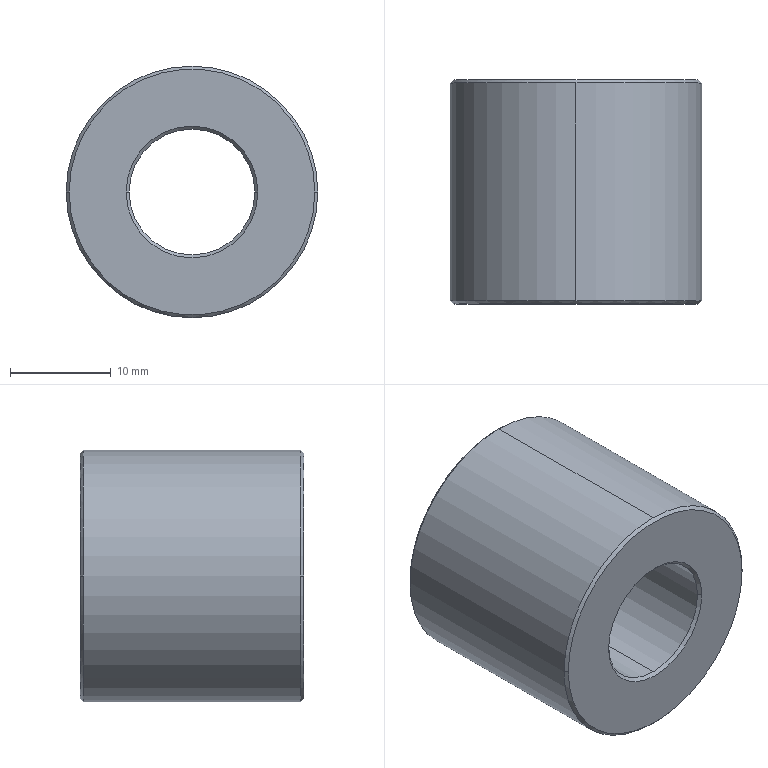Part | NX | 1 solid | 14 faces | box 25 x 22.25 x 25 mm | volume 8181 mm3 | cone 8 | cylinder 4 | plane 2 | commonest cylinder face diameters 12.5 x2 25 x2
STEP:
#1=CARTESIAN_POINT('',(12.5,-29.95,-71.));
#2=VERTEX_POINT('',#1);
#3=CARTESIAN_POINT('',(0.,-29.95,-83.5));
#4=VERTEX_POINT('',#3);
#5=CARTESIAN_POINT('',(0.,-29.95,-71.));
#6=DIRECTION('',(0.,1.,0.));
#7=DIRECTION('',(0.,0.,-1.));
#8=AXIS2_PLACEMENT_3D('',#5,#6,#7);
#9=CIRCLE('',#8,12.5);
#10=EDGE_CURVE('',#2,#4,#9,.T.);
#11=ORIENTED_EDGE('',*,*,#10,.T.);
#12=CARTESIAN_POINT('',(0.,-8.3,-83.5));
#13=VERTEX_POINT('',#12);
#14=CARTESIAN_POINT('',(0.,-30.25,-83.5));
#15=DIRECTION('',(0.,1.,0.));
#16=VECTOR('',#15,1000.);
#17=LINE('',#14,#16);
#18=EDGE_CURVE('',#13,#4,#17,.F.);
#19=ORIENTED_EDGE('',*,*,#18,.F.);
#20=CARTESIAN_POINT('',(12.5,-8.3,-71.));
#21=VERTEX_POINT('',#20);
#22=CARTESIAN_POINT('',(0.,-8.3,-71.));
#23=DIRECTION('',(0.,1.,0.));
#24=DIRECTION('',(0.,0.,-1.));
#25=AXIS2_PLACEMENT_3D('',#22,#23,#24);
#26=CIRCLE('',#25,12.5);
#27=EDGE_CURVE('',#21,#13,#26,.T.);
#28=ORIENTED_EDGE('',*,*,#27,.F.);
#29=CARTESIAN_POINT('',(0.,-8.3,-58.5));
#30=VERTEX_POINT('',#29);
#31=CARTESIAN_POINT('',(0.,-8.3,-71.));
#32=DIRECTION('',(0.,1.,0.));
#33=DIRECTION('',(0.,0.,-1.));
#34=AXIS2_PLACEMENT_3D('',#31,#32,#33);
#35=CIRCLE('',#34,12.5);
#36=EDGE_CURVE('',#30,#21,#35,.T.);
#37=ORIENTED_EDGE('',*,*,#36,.F.);
#38=CARTESIAN_POINT('',(0.,-29.95,-58.5));
#39=VERTEX_POINT('',#38);
#40=CARTESIAN_POINT('',(0.,-30.25,-58.5));
#41=DIRECTION('',(0.,1.,0.));
#42=VECTOR('',#41,1000.);
#43=LINE('',#40,#42);
#44=EDGE_CURVE('',#30,#39,#43,.F.);
#45=ORIENTED_EDGE('',*,*,#44,.T.);
#46=CARTESIAN_POINT('',(0.,-29.95,-71.));
#47=DIRECTION('',(0.,1.,0.));
#48=DIRECTION('',(0.,0.,-1.));
#49=AXIS2_PLACEMENT_3D('',#46,#47,#48);
#50=CIRCLE('',#49,12.5);
#51=EDGE_CURVE('',#39,#2,#50,.T.);
#52=ORIENTED_EDGE('',*,*,#51,.T.);
#53=EDGE_LOOP('',(#11,#19,#28,#37,#45,#52));
#54=FACE_BOUND('',#53,.T.);
#55=CARTESIAN_POINT('',(0.,-30.25,-71.));
#56=DIRECTION('',(0.,1.,0.));
#57=DIRECTION('',(0.,0.,-1.));
#58=AXIS2_PLACEMENT_3D('',#55,#56,#57);
#59=CYLINDRICAL_SURFACE('',#58,12.5);
#60=ADVANCED_FACE('',(#54),#59,.T.);
#61=ORIENTED_EDGE('',*,*,#10,.F.);
#62=CARTESIAN_POINT('',(12.2,-30.25,-71.));
#63=VERTEX_POINT('',#62);
#64=CARTESIAN_POINT('',(12.2,-30.25,-71.));
#65=DIRECTION('',(0.7071,0.7071,0.));
#66=VECTOR('',#65,1000.);
#67=LINE('',#64,#66);
#68=EDGE_CURVE('',#2,#63,#67,.F.);
#69=ORIENTED_EDGE('',*,*,#68,.T.);
#70=CARTESIAN_POINT('',(-12.2,-30.25,-71.));
#71=VERTEX_POINT('',#70);
#72=CARTESIAN_POINT('',(0.,-30.25,-71.));
#73=DIRECTION('',(0.,1.,0.));
#74=DIRECTION('',(0.,0.,-1.));
#75=AXIS2_PLACEMENT_3D('',#72,#73,#74);
#76=CIRCLE('',#75,12.2);
#77=EDGE_CURVE('',#63,#71,#76,.T.);
#78=ORIENTED_EDGE('',*,*,#77,.T.);
#79=CARTESIAN_POINT('',(-12.5,-29.95,-71.));
#80=VERTEX_POINT('',#79);
#81=CARTESIAN_POINT('',(-12.2,-30.25,-71.));
#82=DIRECTION('',(-0.7071,0.7071,0.));
#83=VECTOR('',#82,1000.);
#84=LINE('',#81,#83);
#85=EDGE_CURVE('',#80,#71,#84,.F.);
#86=ORIENTED_EDGE('',*,*,#85,.F.);
#87=CARTESIAN_POINT('',(0.,-29.95,-71.));
#88=DIRECTION('',(0.,1.,0.));
#89=DIRECTION('',(0.,0.,-1.));
#90=AXIS2_PLACEMENT_3D('',#87,#88,#89);
#91=CIRCLE('',#90,12.5);
#92=EDGE_CURVE('',#4,#80,#91,.T.);
#93=ORIENTED_EDGE('',*,*,#92,.F.);
#94=EDGE_LOOP('',(#61,#69,#78,#86,#93));
#95=FACE_BOUND('',#94,.T.);
#96=CARTESIAN_POINT('',(0.,-30.25,-71.));
#97=DIRECTION('',(0.,1.,0.));
#98=DIRECTION('',(1.,0.,0.));
#99=AXIS2_PLACEMENT_3D('',#96,#97,#98);
#100=CONICAL_SURFACE('',#99,12.2,0.7854);
#101=ADVANCED_FACE('',(#95),#100,.T.);
#102=CARTESIAN_POINT('',(6.25,-8.3,-71.));
#103=VERTEX_POINT('',#102);
#104=CARTESIAN_POINT('',(0.,-8.3,-77.25));
#105=VERTEX_POINT('',#104);
#106=CARTESIAN_POINT('',(0.,-8.3,-71.));
#107=DIRECTION('',(0.,1.,0.));
#108=DIRECTION('',(0.,0.,-1.));
#109=AXIS2_PLACEMENT_3D('',#106,#107,#108);
#110=CIRCLE('',#109,6.25);
#111=EDGE_CURVE('',#103,#105,#110,.T.);
#112=ORIENTED_EDGE('',*,*,#111,.T.);
#113=CARTESIAN_POINT('',(0.,-29.95,-77.25));
#114=VERTEX_POINT('',#113);
#115=CARTESIAN_POINT('',(0.,-30.25,-77.25));
#116=DIRECTION('',(0.,1.,0.));
#117=VECTOR('',#116,1000.);
#118=LINE('',#115,#117);
#119=EDGE_CURVE('',#105,#114,#118,.F.);
#120=ORIENTED_EDGE('',*,*,#119,.T.);
#121=CARTESIAN_POINT('',(6.25,-29.95,-71.));
#122=VERTEX_POINT('',#121);
#123=CARTESIAN_POINT('',(0.,-29.95,-71.));
#124=DIRECTION('',(0.,1.,0.));
#125=DIRECTION('',(0.,0.,-1.));
#126=AXIS2_PLACEMENT_3D('',#123,#124,#125);
#127=CIRCLE('',#126,6.25);
#128=EDGE_CURVE('',#122,#114,#127,.T.);
#129=ORIENTED_EDGE('',*,*,#128,.F.);
#130=CARTESIAN_POINT('',(0.,-29.95,-64.75));
#131=VERTEX_POINT('',#130);
#132=CARTESIAN_POINT('',(0.,-29.95,-71.));
#133=DIRECTION('',(0.,1.,0.));
#134=DIRECTION('',(0.,0.,-1.));
#135=AXIS2_PLACEMENT_3D('',#132,#133,#134);
#136=CIRCLE('',#135,6.25);
#137=EDGE_CURVE('',#131,#122,#136,.T.);
#138=ORIENTED_EDGE('',*,*,#137,.F.);
#139=CARTESIAN_POINT('',(0.,-8.3,-64.75));
#140=VERTEX_POINT('',#139);
#141=CARTESIAN_POINT('',(0.,-30.25,-64.75));
#142=DIRECTION('',(0.,1.,0.));
#143=VECTOR('',#142,1000.);
#144=LINE('',#141,#143);
#145=EDGE_CURVE('',#140,#131,#144,.F.);
#146=ORIENTED_EDGE('',*,*,#145,.F.);
#147=CARTESIAN_POINT('',(0.,-8.3,-71.));
#148=DIRECTION('',(0.,1.,0.));
#149=DIRECTION('',(0.,0.,-1.));
#150=AXIS2_PLACEMENT_3D('',#147,#148,#149);
#151=CIRCLE('',#150,6.25);
#152=EDGE_CURVE('',#140,#103,#151,.T.);
#153=ORIENTED_EDGE('',*,*,#152,.T.);
#154=EDGE_LOOP('',(#112,#120,#129,#138,#146,#153));
#155=FACE_BOUND('',#154,.T.);
#156=CARTESIAN_POINT('',(0.,-30.25,-71.));
#157=DIRECTION('',(0.,1.,0.));
#158=DIRECTION('',(0.,0.,-1.));
#159=AXIS2_PLACEMENT_3D('',#156,#157,#158);
#160=CYLINDRICAL_SURFACE('',#159,6.25);
#161=ADVANCED_FACE('',(#155),#160,.F.);
#162=CARTESIAN_POINT('',(-6.25,-29.95,-71.));
#163=VERTEX_POINT('',#162);
#164=CARTESIAN_POINT('',(0.,-29.95,-71.));
#165=DIRECTION('',(0.,1.,0.));
#166=DIRECTION('',(0.,0.,-1.));
#167=AXIS2_PLACEMENT_3D('',#164,#165,#166);
#168=CIRCLE('',#167,6.25);
#169=EDGE_CURVE('',#114,#163,#168,.T.);
#170=ORIENTED_EDGE('',*,*,#169,.T.);
#171=CARTESIAN_POINT('',(-6.55,-30.25,-71.));
#172=VERTEX_POINT('',#171);
#173=CARTESIAN_POINT('',(-6.55,-30.25,-71.));
#174=DIRECTION('',(-0.7071,-0.7071,0.));
#175=VECTOR('',#174,1000.);
#176=LINE('',#173,#175);
#177=EDGE_CURVE('',#172,#163,#176,.F.);
#178=ORIENTED_EDGE('',*,*,#177,.F.);
#179=CARTESIAN_POINT('',(6.55,-30.25,-71.));
#180=VERTEX_POINT('',#179);
#181=CARTESIAN_POINT('',(0.,-30.25,-71.));
#182=DIRECTION('',(0.,1.,0.));
#183=DIRECTION('',(0.,0.,-1.));
#184=AXIS2_PLACEMENT_3D('',#181,#182,#183);
#185=CIRCLE('',#184,6.55);
#186=EDGE_CURVE('',#180,#172,#185,.T.);
#187=ORIENTED_EDGE('',*,*,#186,.F.);
#188=CARTESIAN_POINT('',(6.55,-30.25,-71.));
#189=DIRECTION('',(0.7071,-0.7071,0.));
#190=VECTOR('',#189,1000.);
#191=LINE('',#188,#190);
#192=EDGE_CURVE('',#180,#122,#191,.F.);
#193=ORIENTED_EDGE('',*,*,#192,.T.);
#194=ORIENTED_EDGE('',*,*,#128,.T.);
#195=EDGE_LOOP('',(#170,#178,#187,#193,#194));
#196=FACE_BOUND('',#195,.T.);
#197=CARTESIAN_POINT('',(0.,-30.25,-71.));
#198=DIRECTION('',(0.,-1.,0.));
#199=DIRECTION('',(-1.,0.,0.));
#200=AXIS2_PLACEMENT_3D('',#197,#198,#199);
#201=CONICAL_SURFACE('',#200,6.55,0.7854);
#202=ADVANCED_FACE('',(#196),#201,.F.);
#203=CARTESIAN_POINT('',(-12.2,-8.,-71.));
#204=VERTEX_POINT('',#203);
#205=CARTESIAN_POINT('',(12.2,-8.,-71.));
#206=VERTEX_POINT('',#205);
#207=CARTESIAN_POINT('',(0.,-8.,-71.));
#208=DIRECTION('',(0.,1.,0.));
#209=DIRECTION('',(0.,0.,-1.));
#210=AXIS2_PLACEMENT_3D('',#207,#208,#209);
#211=CIRCLE('',#210,12.2);
#212=EDGE_CURVE('',#204,#206,#211,.T.);
#213=ORIENTED_EDGE('',*,*,#212,.T.);
#214=CARTESIAN_POINT('',(0.,-8.,-71.));
#215=DIRECTION('',(0.,1.,0.));
#216=DIRECTION('',(0.,0.,-1.));
#217=AXIS2_PLACEMENT_3D('',#214,#215,#216);
#218=CIRCLE('',#217,12.2);
#219=EDGE_CURVE('',#206,#204,#218,.T.);
#220=ORIENTED_EDGE('',*,*,#219,.T.);
#221=EDGE_LOOP('',(#213,#220));
#222=FACE_BOUND('',#221,.T.);
#223=CARTESIAN_POINT('',(-6.55,-8.,-71.));
#224=VERTEX_POINT('',#223);
#225=CARTESIAN_POINT('',(6.55,-8.,-71.));
#226=VERTEX_POINT('',#225);
#227=CARTESIAN_POINT('',(0.,-8.,-71.));
#228=DIRECTION('',(0.,1.,0.));
#229=DIRECTION('',(0.,0.,-1.));
#230=AXIS2_PLACEMENT_3D('',#227,#228,#229);
#231=CIRCLE('',#230,6.55);
#232=EDGE_CURVE('',#224,#226,#231,.T.);
#233=ORIENTED_EDGE('',*,*,#232,.F.);
#234=CARTESIAN_POINT('',(0.,-8.,-71.));
#235=DIRECTION('',(0.,1.,0.));
#236=DIRECTION('',(0.,0.,-1.));
#237=AXIS2_PLACEMENT_3D('',#234,#235,#236);
#238=CIRCLE('',#237,6.55);
#239=EDGE_CURVE('',#226,#224,#238,.T.);
#240=ORIENTED_EDGE('',*,*,#239,.F.);
#241=EDGE_LOOP('',(#233,#240));
#242=FACE_BOUND('',#241,.T.);
#243=CARTESIAN_POINT('',(-14.326,-8.,-76.447));
#244=DIRECTION('',(0.,1.,0.));
#245=DIRECTION('',(0.,0.,-1.));
#246=AXIS2_PLACEMENT_3D('',#243,#244,#245);
#247=PLANE('',#246);
#248=ADVANCED_FACE('',(#222,#242),#247,.T.);
#249=ORIENTED_EDGE('',*,*,#212,.F.);
#250=CARTESIAN_POINT('',(-12.5,-8.3,-71.));
#251=VERTEX_POINT('',#250);
#252=CARTESIAN_POINT('',(-12.2,-8.,-71.));
#253=DIRECTION('',(-0.7071,-0.7071,0.));
#254=VECTOR('',#253,1000.);
#255=LINE('',#252,#254);
#256=EDGE_CURVE('',#251,#204,#255,.F.);
#257=ORIENTED_EDGE('',*,*,#256,.F.);
#258=CARTESIAN_POINT('',(0.,-8.3,-71.));
#259=DIRECTION('',(0.,1.,0.));
#260=DIRECTION('',(0.,0.,-1.));
#261=AXIS2_PLACEMENT_3D('',#258,#259,#260);
#262=CIRCLE('',#261,12.5);
#263=EDGE_CURVE('',#251,#30,#262,.T.);
#264=ORIENTED_EDGE('',*,*,#263,.T.);
#265=ORIENTED_EDGE('',*,*,#36,.T.);
#266=CARTESIAN_POINT('',(12.2,-8.,-71.));
#267=DIRECTION('',(0.7071,-0.7071,0.));
#268=VECTOR('',#267,1000.);
#269=LINE('',#266,#268);
#270=EDGE_CURVE('',#21,#206,#269,.F.);
#271=ORIENTED_EDGE('',*,*,#270,.T.);
#272=EDGE_LOOP('',(#249,#257,#264,#265,#271));
#273=FACE_BOUND('',#272,.T.);
#274=CARTESIAN_POINT('',(0.,-8.,-71.));
#275=DIRECTION('',(0.,-1.,0.));
#276=DIRECTION('',(-1.,0.,0.));
#277=AXIS2_PLACEMENT_3D('',#274,#275,#276);
#278=CONICAL_SURFACE('',#277,12.2,0.7854);
#279=ADVANCED_FACE('',(#273),#278,.T.);
#280=ORIENTED_EDGE('',*,*,#111,.F.);
#281=CARTESIAN_POINT('',(6.55,-8.,-71.));
#282=DIRECTION('',(0.7071,0.7071,0.));
#283=VECTOR('',#282,1000.);
#284=LINE('',#281,#283);
#285=EDGE_CURVE('',#103,#226,#284,.T.);
#286=ORIENTED_EDGE('',*,*,#285,.T.);
#287=ORIENTED_EDGE('',*,*,#239,.T.);
#288=CARTESIAN_POINT('',(-6.25,-8.3,-71.));
#289=VERTEX_POINT('',#288);
#290=CARTESIAN_POINT('',(-6.55,-8.,-71.));
#291=DIRECTION('',(-0.7071,0.7071,0.));
#292=VECTOR('',#291,1000.);
#293=LINE('',#290,#292);
#294=EDGE_CURVE('',#289,#224,#293,.T.);
#295=ORIENTED_EDGE('',*,*,#294,.F.);
#296=CARTESIAN_POINT('',(0.,-8.3,-71.));
#297=DIRECTION('',(0.,1.,0.));
#298=DIRECTION('',(0.,0.,-1.));
#299=AXIS2_PLACEMENT_3D('',#296,#297,#298);
#300=CIRCLE('',#299,6.25);
#301=EDGE_CURVE('',#105,#289,#300,.T.);
#302=ORIENTED_EDGE('',*,*,#301,.F.);
#303=EDGE_LOOP('',(#280,#286,#287,#295,#302));
#304=FACE_BOUND('',#303,.T.);
#305=CARTESIAN_POINT('',(0.,-8.,-71.));
#306=DIRECTION('',(0.,1.,0.));
#307=DIRECTION('',(1.,0.,0.));
#308=AXIS2_PLACEMENT_3D('',#305,#306,#307);
#309=CONICAL_SURFACE('',#308,6.55,0.7854);
#310=ADVANCED_FACE('',(#304),#309,.F.);
#311=ORIENTED_EDGE('',*,*,#77,.F.);
#312=CARTESIAN_POINT('',(0.,-30.25,-71.));
#313=DIRECTION('',(0.,1.,0.));
#314=DIRECTION('',(0.,0.,-1.));
#315=AXIS2_PLACEMENT_3D('',#312,#313,#314);
#316=CIRCLE('',#315,12.2);
#317=EDGE_CURVE('',#71,#63,#316,.T.);
#318=ORIENTED_EDGE('',*,*,#317,.F.);
#319=EDGE_LOOP('',(#311,#318));
#320=FACE_BOUND('',#319,.T.);
#321=CARTESIAN_POINT('',(0.,-30.25,-71.));
#322=DIRECTION('',(0.,1.,0.));
#323=DIRECTION('',(0.,0.,-1.));
#324=AXIS2_PLACEMENT_3D('',#321,#322,#323);
#325=CIRCLE('',#324,6.55);
#326=EDGE_CURVE('',#172,#180,#325,.T.);
#327=ORIENTED_EDGE('',*,*,#326,.T.);
#328=ORIENTED_EDGE('',*,*,#186,.T.);
#329=EDGE_LOOP('',(#327,#328));
#330=FACE_BOUND('',#329,.T.);
#331=CARTESIAN_POINT('',(-14.326,-30.25,-76.447));
#332=DIRECTION('',(0.,1.,0.));
#333=DIRECTION('',(0.,0.,-1.));
#334=AXIS2_PLACEMENT_3D('',#331,#332,#333);
#335=PLANE('',#334);
#336=ADVANCED_FACE('',(#320,#330),#335,.F.);
#337=CARTESIAN_POINT('',(0.,-8.3,-71.));
#338=DIRECTION('',(0.,1.,0.));
#339=DIRECTION('',(0.,0.,-1.));
#340=AXIS2_PLACEMENT_3D('',#337,#338,#339);
#341=CIRCLE('',#340,12.5);
#342=EDGE_CURVE('',#13,#251,#341,.T.);
#343=ORIENTED_EDGE('',*,*,#342,.T.);
#344=ORIENTED_EDGE('',*,*,#256,.T.);
#345=ORIENTED_EDGE('',*,*,#219,.F.);
#346=ORIENTED_EDGE('',*,*,#270,.F.);
#347=ORIENTED_EDGE('',*,*,#27,.T.);
#348=EDGE_LOOP('',(#343,#344,#345,#346,#347));
#349=FACE_BOUND('',#348,.T.);
#350=CARTESIAN_POINT('',(0.,-8.,-71.));
#351=DIRECTION('',(0.,-1.,0.));
#352=DIRECTION('',(-1.,0.,0.));
#353=AXIS2_PLACEMENT_3D('',#350,#351,#352);
#354=CONICAL_SURFACE('',#353,12.2,0.7854);
#355=ADVANCED_FACE('',(#349),#354,.T.);
#356=ORIENTED_EDGE('',*,*,#342,.F.);
#357=ORIENTED_EDGE('',*,*,#18,.T.);
#358=ORIENTED_EDGE('',*,*,#92,.T.);
#359=CARTESIAN_POINT('',(0.,-29.95,-71.));
#360=DIRECTION('',(0.,1.,0.));
#361=DIRECTION('',(0.,0.,-1.));
#362=AXIS2_PLACEMENT_3D('',#359,#360,#361);
#363=CIRCLE('',#362,12.5);
#364=EDGE_CURVE('',#80,#39,#363,.T.);
#365=ORIENTED_EDGE('',*,*,#364,.T.);
#366=ORIENTED_EDGE('',*,*,#44,.F.);
#367=ORIENTED_EDGE('',*,*,#263,.F.);
#368=EDGE_LOOP('',(#356,#357,#358,#365,#366,#367));
#369=FACE_BOUND('',#368,.T.);
#370=CARTESIAN_POINT('',(0.,-30.25,-71.));
#371=DIRECTION('',(0.,1.,0.));
#372=DIRECTION('',(0.,0.,-1.));
#373=AXIS2_PLACEMENT_3D('',#370,#371,#372);
#374=CYLINDRICAL_SURFACE('',#373,12.5);
#375=ADVANCED_FACE('',(#369),#374,.T.);
#376=ORIENTED_EDGE('',*,*,#232,.T.);
#377=ORIENTED_EDGE('',*,*,#285,.F.);
#378=ORIENTED_EDGE('',*,*,#152,.F.);
#379=CARTESIAN_POINT('',(0.,-8.3,-71.));
#380=DIRECTION('',(0.,1.,0.));
#381=DIRECTION('',(0.,0.,-1.));
#382=AXIS2_PLACEMENT_3D('',#379,#380,#381);
#383=CIRCLE('',#382,6.25);
#384=EDGE_CURVE('',#289,#140,#383,.T.);
#385=ORIENTED_EDGE('',*,*,#384,.F.);
#386=ORIENTED_EDGE('',*,*,#294,.T.);
#387=EDGE_LOOP('',(#376,#377,#378,#385,#386));
#388=FACE_BOUND('',#387,.T.);
#389=CARTESIAN_POINT('',(0.,-8.,-71.));
#390=DIRECTION('',(0.,1.,0.));
#391=DIRECTION('',(1.,0.,0.));
#392=AXIS2_PLACEMENT_3D('',#389,#390,#391);
#393=CONICAL_SURFACE('',#392,6.55,0.7854);
#394=ADVANCED_FACE('',(#388),#393,.F.);
#395=ORIENTED_EDGE('',*,*,#169,.F.);
#396=ORIENTED_EDGE('',*,*,#119,.F.);
#397=ORIENTED_EDGE('',*,*,#301,.T.);
#398=ORIENTED_EDGE('',*,*,#384,.T.);
#399=ORIENTED_EDGE('',*,*,#145,.T.);
#400=CARTESIAN_POINT('',(0.,-29.95,-71.));
#401=DIRECTION('',(0.,1.,0.));
#402=DIRECTION('',(0.,0.,-1.));
#403=AXIS2_PLACEMENT_3D('',#400,#401,#402);
#404=CIRCLE('',#403,6.25);
#405=EDGE_CURVE('',#163,#131,#404,.T.);
#406=ORIENTED_EDGE('',*,*,#405,.F.);
#407=EDGE_LOOP('',(#395,#396,#397,#398,#399,#406));
#408=FACE_BOUND('',#407,.T.);
#409=CARTESIAN_POINT('',(0.,-30.25,-71.));
#410=DIRECTION('',(0.,1.,0.));
#411=DIRECTION('',(0.,0.,-1.));
#412=AXIS2_PLACEMENT_3D('',#409,#410,#411);
#413=CYLINDRICAL_SURFACE('',#412,6.25);
#414=ADVANCED_FACE('',(#408),#413,.F.);
#415=ORIENTED_EDGE('',*,*,#177,.T.);
#416=ORIENTED_EDGE('',*,*,#405,.T.);
#417=ORIENTED_EDGE('',*,*,#137,.T.);
#418=ORIENTED_EDGE('',*,*,#192,.F.);
#419=ORIENTED_EDGE('',*,*,#326,.F.);
#420=EDGE_LOOP('',(#415,#416,#417,#418,#419));
#421=FACE_BOUND('',#420,.T.);
#422=CARTESIAN_POINT('',(0.,-30.25,-71.));
#423=DIRECTION('',(0.,-1.,0.));
#424=DIRECTION('',(-1.,0.,0.));
#425=AXIS2_PLACEMENT_3D('',#422,#423,#424);
#426=CONICAL_SURFACE('',#425,6.55,0.7854);
#427=ADVANCED_FACE('',(#421),#426,.F.);
#428=ORIENTED_EDGE('',*,*,#85,.T.);
#429=ORIENTED_EDGE('',*,*,#317,.T.);
#430=ORIENTED_EDGE('',*,*,#68,.F.);
#431=ORIENTED_EDGE('',*,*,#51,.F.);
#432=ORIENTED_EDGE('',*,*,#364,.F.);
#433=EDGE_LOOP('',(#428,#429,#430,#431,#432));
#434=FACE_BOUND('',#433,.T.);
#435=CARTESIAN_POINT('',(0.,-30.25,-71.));
#436=DIRECTION('',(0.,1.,0.));
#437=DIRECTION('',(1.,0.,0.));
#438=AXIS2_PLACEMENT_3D('',#435,#436,#437);
#439=CONICAL_SURFACE('',#438,12.2,0.7854);
#440=ADVANCED_FACE('',(#434),#439,.T.);
#441=CLOSED_SHELL('',(#60,#101,#161,#202,#248,#279,#310,#336,#355,#375,#394,#414,#427,#440));
#442=MANIFOLD_SOLID_BREP('',#441);
#443=(LENGTH_UNIT()NAMED_UNIT(*)SI_UNIT(.MILLI.,.METRE.));
#444=UNCERTAINTY_MEASURE_WITH_UNIT(LENGTH_MEASURE(0.00001),#443,'','');
#445=(NAMED_UNIT(*)PLANE_ANGLE_UNIT()SI_UNIT($,.RADIAN.));
#446=(NAMED_UNIT(*)SI_UNIT($,.STERADIAN.)SOLID_ANGLE_UNIT());
#447=(GEOMETRIC_REPRESENTATION_CONTEXT(3)GLOBAL_UNCERTAINTY_ASSIGNED_CONTEXT((#444))GLOBAL_UNIT_ASSIGNED_CONTEXT((#443,#445,#446))REPRESENTATION_CONTEXT('',''));
#448=ADVANCED_BREP_SHAPE_REPRESENTATION('',(#442),#447);